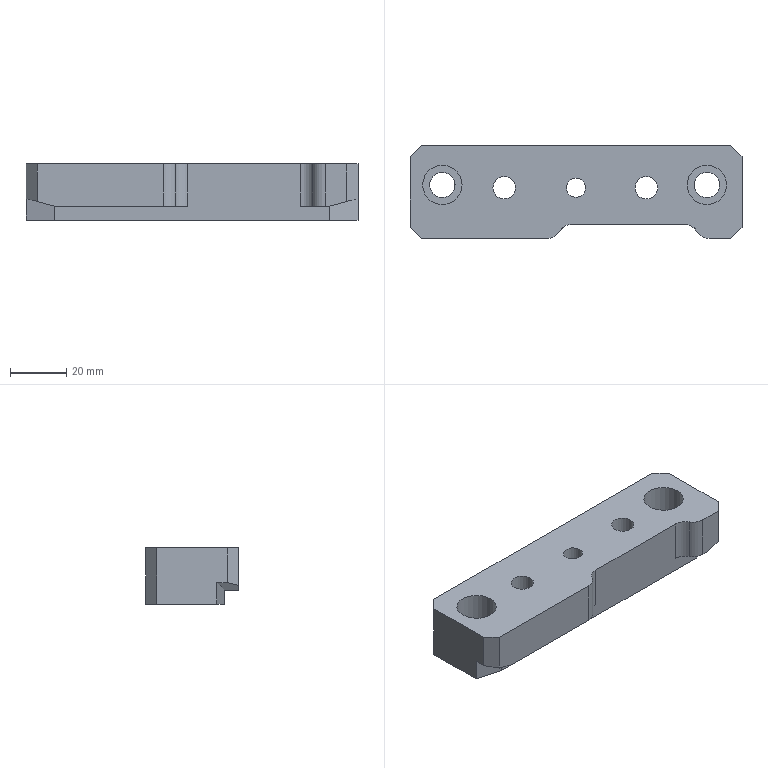Part | NX | features 20 2 | 1 solid | 31 faces | box 118 x 33 x 20 mm | volume 63338 mm3 | plane 20 | cylinder 11 | commonest cylinder face diameters 10 x4 8.001 x2 9 x2 14 x2 6.8 x1
STEP:
#1=CARTESIAN_POINT('',(771.502,417.5,1.5));
#2=VERTEX_POINT('',#1);
#3=CARTESIAN_POINT('',(771.502,422.5,1.5));
#4=VERTEX_POINT('',#3);
#5=CARTESIAN_POINT('',(771.502,417.5,1.5));
#6=DIRECTION('',(0.,1.,0.));
#7=VECTOR('',#6,1000.);
#8=LINE('',#5,#7);
#9=EDGE_CURVE('',#2,#4,#8,.T.);
#10=ORIENTED_EDGE('',*,*,#9,.T.);
#11=CARTESIAN_POINT('',(818.929,422.5,1.5));
#12=VERTEX_POINT('',#11);
#13=CARTESIAN_POINT('',(698.,422.5,1.5));
#14=DIRECTION('',(-1.,0.,0.));
#15=VECTOR('',#14,1000.);
#16=LINE('',#13,#15);
#17=EDGE_CURVE('',#12,#4,#16,.T.);
#18=ORIENTED_EDGE('',*,*,#17,.F.);
#19=CARTESIAN_POINT('',(814.598,420.,1.5));
#20=VERTEX_POINT('',#19);
#21=CARTESIAN_POINT('',(818.929,417.5,1.5));
#22=DIRECTION('',(0.,0.,-1.));
#23=DIRECTION('',(-1.,0.,0.));
#24=AXIS2_PLACEMENT_3D('',#21,#22,#23);
#25=CIRCLE('',#24,5.);
#26=EDGE_CURVE('',#20,#12,#25,.T.);
#27=ORIENTED_EDGE('',*,*,#26,.F.);
#28=CARTESIAN_POINT('',(810.268,417.5,1.5));
#29=VERTEX_POINT('',#28);
#30=CARTESIAN_POINT('',(810.268,422.5,1.5));
#31=DIRECTION('',(0.,0.,-1.));
#32=DIRECTION('',(-1.,0.,0.));
#33=AXIS2_PLACEMENT_3D('',#30,#31,#32);
#34=CIRCLE('',#33,5.);
#35=EDGE_CURVE('',#20,#29,#34,.T.);
#36=ORIENTED_EDGE('',*,*,#35,.T.);
#37=CARTESIAN_POINT('',(708.002,417.5,1.5));
#38=DIRECTION('',(-1.,0.,0.));
#39=VECTOR('',#38,1000.);
#40=LINE('',#37,#39);
#41=EDGE_CURVE('',#29,#2,#40,.T.);
#42=ORIENTED_EDGE('',*,*,#41,.T.);
#43=EDGE_LOOP('',(#10,#18,#27,#36,#42));
#44=FACE_BOUND('',#43,.T.);
#45=CARTESIAN_POINT('',(730.272,396.891,1.5));
#46=DIRECTION('',(0.,0.,-1.));
#47=DIRECTION('',(1.,0.,0.));
#48=AXIS2_PLACEMENT_3D('',#45,#46,#47);
#49=PLANE('',#48);
#50=ADVANCED_FACE('',(#44),#49,.T.);
#51=CARTESIAN_POINT('',(863.459,420.,1.5));
#52=VERTEX_POINT('',#51);
#53=CARTESIAN_POINT('',(859.129,422.5,1.5));
#54=VERTEX_POINT('',#53);
#55=CARTESIAN_POINT('',(859.129,417.5,1.5));
#56=DIRECTION('',(0.,0.,1.));
#57=DIRECTION('',(-1.,0.,0.));
#58=AXIS2_PLACEMENT_3D('',#55,#56,#57);
#59=CIRCLE('',#58,5.);
#60=EDGE_CURVE('',#52,#54,#59,.T.);
#61=ORIENTED_EDGE('',*,*,#60,.T.);
#62=CARTESIAN_POINT('',(869.503,422.5,1.5));
#63=VERTEX_POINT('',#62);
#64=CARTESIAN_POINT('',(698.,422.5,1.5));
#65=DIRECTION('',(-1.,0.,0.));
#66=VECTOR('',#65,1000.);
#67=LINE('',#64,#66);
#68=EDGE_CURVE('',#63,#54,#67,.T.);
#69=ORIENTED_EDGE('',*,*,#68,.F.);
#70=CARTESIAN_POINT('',(869.502,422.5,1.5));
#71=VERTEX_POINT('',#70);
#72=CARTESIAN_POINT('',(733.197,385.977,1.5));
#73=DIRECTION('',(0.9659,0.2588,0.));
#74=VECTOR('',#73,1000.);
#75=LINE('',#72,#74);
#76=EDGE_CURVE('',#71,#63,#75,.T.);
#77=ORIENTED_EDGE('',*,*,#76,.F.);
#78=CARTESIAN_POINT('',(869.502,417.5,1.5));
#79=VERTEX_POINT('',#78);
#80=CARTESIAN_POINT('',(869.502,396.891,1.5));
#81=DIRECTION('',(0.,1.,0.));
#82=VECTOR('',#81,1000.);
#83=LINE('',#80,#82);
#84=EDGE_CURVE('',#79,#71,#83,.T.);
#85=ORIENTED_EDGE('',*,*,#84,.F.);
#86=CARTESIAN_POINT('',(867.789,417.5,1.5));
#87=VERTEX_POINT('',#86);
#88=CARTESIAN_POINT('',(689.002,417.5,1.5));
#89=DIRECTION('',(-1.,0.,0.));
#90=VECTOR('',#89,1000.);
#91=LINE('',#88,#90);
#92=EDGE_CURVE('',#79,#87,#91,.T.);
#93=ORIENTED_EDGE('',*,*,#92,.T.);
#94=CARTESIAN_POINT('',(867.789,422.5,1.5));
#95=DIRECTION('',(0.,0.,1.));
#96=DIRECTION('',(-1.,0.,0.));
#97=AXIS2_PLACEMENT_3D('',#94,#95,#96);
#98=CIRCLE('',#97,5.);
#99=EDGE_CURVE('',#52,#87,#98,.T.);
#100=ORIENTED_EDGE('',*,*,#99,.F.);
#101=EDGE_LOOP('',(#61,#69,#77,#85,#93,#100));
#102=FACE_BOUND('',#101,.T.);
#103=CARTESIAN_POINT('',(730.272,396.891,1.5));
#104=DIRECTION('',(0.,0.,-1.));
#105=DIRECTION('',(1.,0.,0.));
#106=AXIS2_PLACEMENT_3D('',#103,#104,#105);
#107=PLANE('',#106);
#108=ADVANCED_FACE('',(#102),#107,.T.);
#109=CARTESIAN_POINT('',(875.502,417.5,3.108));
#110=VERTEX_POINT('',#109);
#111=CARTESIAN_POINT('',(869.502,417.5,1.5));
#112=DIRECTION('',(0.9659,0.,0.2588));
#113=VECTOR('',#112,1000.);
#114=LINE('',#111,#113);
#115=EDGE_CURVE('',#79,#110,#114,.T.);
#116=ORIENTED_EDGE('',*,*,#115,.F.);
#117=ORIENTED_EDGE('',*,*,#84,.T.);
#118=CARTESIAN_POINT('',(879.502,425.179,4.179));
#119=VERTEX_POINT('',#118);
#120=CARTESIAN_POINT('',(869.971,422.626,1.626));
#121=DIRECTION('',(-0.9351,-0.2506,-0.2506));
#122=VECTOR('',#121,1000.);
#123=LINE('',#120,#122);
#124=EDGE_CURVE('',#119,#71,#123,.T.);
#125=ORIENTED_EDGE('',*,*,#124,.F.);
#126=CARTESIAN_POINT('',(879.502,421.5,4.179));
#127=VERTEX_POINT('',#126);
#128=CARTESIAN_POINT('',(879.502,396.891,4.179));
#129=DIRECTION('',(0.,1.,0.));
#130=VECTOR('',#129,1000.);
#131=LINE('',#128,#130);
#132=EDGE_CURVE('',#127,#119,#131,.T.);
#133=ORIENTED_EDGE('',*,*,#132,.F.);
#134=CARTESIAN_POINT('',(876.587,418.585,3.399));
#135=DIRECTION('',(-0.6947,-0.6947,-0.1862));
#136=VECTOR('',#135,1000.);
#137=LINE('',#134,#136);
#138=EDGE_CURVE('',#127,#110,#137,.T.);
#139=ORIENTED_EDGE('',*,*,#138,.T.);
#140=EDGE_LOOP('',(#116,#117,#125,#133,#139));
#141=FACE_BOUND('',#140,.T.);
#142=CARTESIAN_POINT('',(869.502,396.891,1.5));
#143=DIRECTION('',(0.2588,0.,-0.9659));
#144=DIRECTION('',(-0.9659,0.,-0.2588));
#145=AXIS2_PLACEMENT_3D('',#142,#143,#144);
#146=PLANE('',#145);
#147=ADVANCED_FACE('',(#141),#146,.T.);
#148=CARTESIAN_POINT('',(799.002,435.5,-3.5));
#149=VERTEX_POINT('',#148);
#150=CARTESIAN_POINT('',(795.002,435.5,-3.5));
#151=DIRECTION('',(0.,0.,-1.));
#152=DIRECTION('',(1.,0.,0.));
#153=AXIS2_PLACEMENT_3D('',#150,#151,#152);
#154=CIRCLE('',#153,4.);
#155=EDGE_CURVE('',#149,#149,#154,.T.);
#156=ORIENTED_EDGE('',*,*,#155,.T.);
#157=EDGE_LOOP('',(#156));
#158=FACE_BOUND('',#157,.T.);
#159=CARTESIAN_POINT('',(799.002,435.5,16.5));
#160=VERTEX_POINT('',#159);
#161=CARTESIAN_POINT('',(795.002,435.5,16.5));
#162=DIRECTION('',(0.,0.,1.));
#163=DIRECTION('',(1.,0.,0.));
#164=AXIS2_PLACEMENT_3D('',#161,#162,#163);
#165=CIRCLE('',#164,4.);
#166=EDGE_CURVE('',#160,#160,#165,.T.);
#167=ORIENTED_EDGE('',*,*,#166,.T.);
#168=EDGE_LOOP('',(#167));
#169=FACE_BOUND('',#168,.T.);
#170=CARTESIAN_POINT('',(795.002,435.5,42.5));
#171=DIRECTION('',(0.,0.,-1.));
#172=DIRECTION('',(1.,0.,0.));
#173=AXIS2_PLACEMENT_3D('',#170,#171,#172);
#174=CYLINDRICAL_SURFACE('',#173,4.);
#175=ADVANCED_FACE('',(#158,#169),#174,.F.);
#176=CARTESIAN_POINT('',(849.502,435.5,-3.5));
#177=VERTEX_POINT('',#176);
#178=CARTESIAN_POINT('',(845.502,435.5,-3.5));
#179=DIRECTION('',(0.,0.,1.));
#180=DIRECTION('',(1.,0.,0.));
#181=AXIS2_PLACEMENT_3D('',#178,#179,#180);
#182=CIRCLE('',#181,4.);
#183=EDGE_CURVE('',#177,#177,#182,.T.);
#184=ORIENTED_EDGE('',*,*,#183,.F.);
#185=EDGE_LOOP('',(#184));
#186=FACE_BOUND('',#185,.T.);
#187=CARTESIAN_POINT('',(849.502,435.5,16.5));
#188=VERTEX_POINT('',#187);
#189=CARTESIAN_POINT('',(845.502,435.5,16.5));
#190=DIRECTION('',(0.,0.,1.));
#191=DIRECTION('',(1.,0.,0.));
#192=AXIS2_PLACEMENT_3D('',#189,#190,#191);
#193=CIRCLE('',#192,4.);
#194=EDGE_CURVE('',#188,#188,#193,.T.);
#195=ORIENTED_EDGE('',*,*,#194,.T.);
#196=EDGE_LOOP('',(#195));
#197=FACE_BOUND('',#196,.T.);
#198=CARTESIAN_POINT('',(845.502,435.5,42.5));
#199=DIRECTION('',(0.,0.,-1.));
#200=DIRECTION('',(1.,0.,0.));
#201=AXIS2_PLACEMENT_3D('',#198,#199,#200);
#202=CYLINDRICAL_SURFACE('',#201,4.);
#203=ADVANCED_FACE('',(#186,#197),#202,.F.);
#204=CARTESIAN_POINT('',(879.502,425.179,-3.5));
#205=VERTEX_POINT('',#204);
#206=CARTESIAN_POINT('',(879.502,425.179,3.5));
#207=DIRECTION('',(0.,0.,1.));
#208=VECTOR('',#207,1000.);
#209=LINE('',#206,#208);
#210=EDGE_CURVE('',#205,#119,#209,.T.);
#211=ORIENTED_EDGE('',*,*,#210,.F.);
#212=CARTESIAN_POINT('',(879.502,446.5,-3.5));
#213=VERTEX_POINT('',#212);
#214=CARTESIAN_POINT('',(879.502,450.5,-3.5));
#215=DIRECTION('',(0.,1.,0.));
#216=VECTOR('',#215,1000.);
#217=LINE('',#214,#216);
#218=EDGE_CURVE('',#205,#213,#217,.T.);
#219=ORIENTED_EDGE('',*,*,#218,.T.);
#220=CARTESIAN_POINT('',(879.502,446.5,16.5));
#221=VERTEX_POINT('',#220);
#222=CARTESIAN_POINT('',(879.502,446.5,11.5));
#223=DIRECTION('',(0.,0.,1.));
#224=VECTOR('',#223,1000.);
#225=LINE('',#222,#224);
#226=EDGE_CURVE('',#213,#221,#225,.T.);
#227=ORIENTED_EDGE('',*,*,#226,.T.);
#228=CARTESIAN_POINT('',(879.502,421.5,16.5));
#229=VERTEX_POINT('',#228);
#230=CARTESIAN_POINT('',(879.502,450.5,16.5));
#231=DIRECTION('',(0.,1.,0.));
#232=VECTOR('',#231,1000.);
#233=LINE('',#230,#232);
#234=EDGE_CURVE('',#229,#221,#233,.T.);
#235=ORIENTED_EDGE('',*,*,#234,.F.);
#236=CARTESIAN_POINT('',(879.502,421.5,11.5));
#237=DIRECTION('',(0.,0.,-1.));
#238=VECTOR('',#237,1000.);
#239=LINE('',#236,#238);
#240=EDGE_CURVE('',#229,#127,#239,.T.);
#241=ORIENTED_EDGE('',*,*,#240,.T.);
#242=ORIENTED_EDGE('',*,*,#132,.T.);
#243=EDGE_LOOP('',(#211,#219,#227,#235,#241,#242));
#244=FACE_BOUND('',#243,.T.);
#245=CARTESIAN_POINT('',(879.502,450.5,11.5));
#246=DIRECTION('',(-1.,0.,0.));
#247=DIRECTION('',(0.,0.,-1.));
#248=AXIS2_PLACEMENT_3D('',#245,#246,#247);
#249=PLANE('',#248);
#250=ADVANCED_FACE('',(#244),#249,.F.);
#251=ORIENTED_EDGE('',*,*,#226,.F.);
#252=CARTESIAN_POINT('',(875.502,450.5,-3.5));
#253=VERTEX_POINT('',#252);
#254=CARTESIAN_POINT('',(879.502,446.5,-3.5));
#255=DIRECTION('',(0.7071,-0.7071,0.));
#256=VECTOR('',#255,1000.);
#257=LINE('',#254,#256);
#258=EDGE_CURVE('',#253,#213,#257,.T.);
#259=ORIENTED_EDGE('',*,*,#258,.F.);
#260=CARTESIAN_POINT('',(875.502,450.5,16.5));
#261=VERTEX_POINT('',#260);
#262=CARTESIAN_POINT('',(875.502,450.5,11.5));
#263=DIRECTION('',(0.,0.,-1.));
#264=VECTOR('',#263,1000.);
#265=LINE('',#262,#264);
#266=EDGE_CURVE('',#261,#253,#265,.T.);
#267=ORIENTED_EDGE('',*,*,#266,.F.);
#268=CARTESIAN_POINT('',(879.502,446.5,16.5));
#269=DIRECTION('',(-0.7071,0.7071,0.));
#270=VECTOR('',#269,1000.);
#271=LINE('',#268,#270);
#272=EDGE_CURVE('',#221,#261,#271,.T.);
#273=ORIENTED_EDGE('',*,*,#272,.F.);
#274=EDGE_LOOP('',(#251,#259,#267,#273));
#275=FACE_BOUND('',#274,.T.);
#276=CARTESIAN_POINT('',(879.502,446.5,11.5));
#277=DIRECTION('',(-0.7071,-0.7071,0.));
#278=DIRECTION('',(0.,0.,-1.));
#279=AXIS2_PLACEMENT_3D('',#276,#277,#278);
#280=PLANE('',#279);
#281=ADVANCED_FACE('',(#275),#280,.F.);
#282=ORIENTED_EDGE('',*,*,#266,.T.);
#283=CARTESIAN_POINT('',(765.502,450.5,-3.5));
#284=VERTEX_POINT('',#283);
#285=CARTESIAN_POINT('',(628.002,450.5,-3.5));
#286=DIRECTION('',(-1.,0.,0.));
#287=VECTOR('',#286,1000.);
#288=LINE('',#285,#287);
#289=EDGE_CURVE('',#253,#284,#288,.T.);
#290=ORIENTED_EDGE('',*,*,#289,.T.);
#291=CARTESIAN_POINT('',(765.502,450.5,16.5));
#292=VERTEX_POINT('',#291);
#293=CARTESIAN_POINT('',(765.502,450.5,11.5));
#294=DIRECTION('',(0.,0.,1.));
#295=VECTOR('',#294,1000.);
#296=LINE('',#293,#295);
#297=EDGE_CURVE('',#284,#292,#296,.T.);
#298=ORIENTED_EDGE('',*,*,#297,.T.);
#299=CARTESIAN_POINT('',(628.002,450.5,16.5));
#300=DIRECTION('',(-1.,0.,0.));
#301=VECTOR('',#300,1000.);
#302=LINE('',#299,#301);
#303=EDGE_CURVE('',#261,#292,#302,.T.);
#304=ORIENTED_EDGE('',*,*,#303,.F.);
#305=EDGE_LOOP('',(#282,#290,#298,#304));
#306=FACE_BOUND('',#305,.T.);
#307=CARTESIAN_POINT('',(628.002,450.5,11.5));
#308=DIRECTION('',(0.,-1.,0.));
#309=DIRECTION('',(0.,0.,-1.));
#310=AXIS2_PLACEMENT_3D('',#307,#308,#309);
#311=PLANE('',#310);
#312=ADVANCED_FACE('',(#306),#311,.F.);
#313=ORIENTED_EDGE('',*,*,#297,.F.);
#314=CARTESIAN_POINT('',(761.502,446.5,-3.5));
#315=VERTEX_POINT('',#314);
#316=CARTESIAN_POINT('',(765.502,450.5,-3.5));
#317=DIRECTION('',(0.7071,0.7071,0.));
#318=VECTOR('',#317,1000.);
#319=LINE('',#316,#318);
#320=EDGE_CURVE('',#315,#284,#319,.T.);
#321=ORIENTED_EDGE('',*,*,#320,.F.);
#322=CARTESIAN_POINT('',(761.502,446.5,16.5));
#323=VERTEX_POINT('',#322);
#324=CARTESIAN_POINT('',(761.502,446.5,11.5));
#325=DIRECTION('',(0.,0.,-1.));
#326=VECTOR('',#325,1000.);
#327=LINE('',#324,#326);
#328=EDGE_CURVE('',#323,#315,#327,.T.);
#329=ORIENTED_EDGE('',*,*,#328,.F.);
#330=CARTESIAN_POINT('',(765.502,450.5,16.5));
#331=DIRECTION('',(-0.7071,-0.7071,0.));
#332=VECTOR('',#331,1000.);
#333=LINE('',#330,#332);
#334=EDGE_CURVE('',#292,#323,#333,.T.);
#335=ORIENTED_EDGE('',*,*,#334,.F.);
#336=EDGE_LOOP('',(#313,#321,#329,#335));
#337=FACE_BOUND('',#336,.T.);
#338=CARTESIAN_POINT('',(765.502,450.5,11.5));
#339=DIRECTION('',(0.7071,-0.7071,0.));
#340=DIRECTION('',(0.,0.,-1.));
#341=AXIS2_PLACEMENT_3D('',#338,#339,#340);
#342=PLANE('',#341);
#343=ADVANCED_FACE('',(#337),#342,.F.);
#344=ORIENTED_EDGE('',*,*,#328,.T.);
#345=CARTESIAN_POINT('',(761.502,425.179,-3.5));
#346=VERTEX_POINT('',#345);
#347=CARTESIAN_POINT('',(761.502,417.5,-3.5));
#348=DIRECTION('',(0.,-1.,0.));
#349=VECTOR('',#348,1000.);
#350=LINE('',#347,#349);
#351=EDGE_CURVE('',#315,#346,#350,.T.);
#352=ORIENTED_EDGE('',*,*,#351,.T.);
#353=CARTESIAN_POINT('',(761.502,425.179,4.179));
#354=VERTEX_POINT('',#353);
#355=CARTESIAN_POINT('',(761.502,425.179,3.5));
#356=DIRECTION('',(0.,0.,1.));
#357=VECTOR('',#356,1000.);
#358=LINE('',#355,#357);
#359=EDGE_CURVE('',#346,#354,#358,.T.);
#360=ORIENTED_EDGE('',*,*,#359,.T.);
#361=CARTESIAN_POINT('',(761.502,421.5,4.179));
#362=VERTEX_POINT('',#361);
#363=CARTESIAN_POINT('',(761.502,425.179,4.179));
#364=DIRECTION('',(0.,-1.,0.));
#365=VECTOR('',#364,1000.);
#366=LINE('',#363,#365);
#367=EDGE_CURVE('',#354,#362,#366,.T.);
#368=ORIENTED_EDGE('',*,*,#367,.T.);
#369=CARTESIAN_POINT('',(761.502,421.5,16.5));
#370=VERTEX_POINT('',#369);
#371=CARTESIAN_POINT('',(761.502,421.5,11.5));
#372=DIRECTION('',(0.,0.,1.));
#373=VECTOR('',#372,1000.);
#374=LINE('',#371,#373);
#375=EDGE_CURVE('',#362,#370,#374,.T.);
#376=ORIENTED_EDGE('',*,*,#375,.T.);
#377=CARTESIAN_POINT('',(761.502,417.5,16.5));
#378=DIRECTION('',(0.,-1.,0.));
#379=VECTOR('',#378,1000.);
#380=LINE('',#377,#379);
#381=EDGE_CURVE('',#323,#370,#380,.T.);
#382=ORIENTED_EDGE('',*,*,#381,.F.);
#383=EDGE_LOOP('',(#344,#352,#360,#368,#376,#382));
#384=FACE_BOUND('',#383,.T.);
#385=CARTESIAN_POINT('',(761.502,417.5,11.5));
#386=DIRECTION('',(1.,0.,0.));
#387=DIRECTION('',(0.,0.,1.));
#388=AXIS2_PLACEMENT_3D('',#385,#386,#387);
#389=PLANE('',#388);
#390=ADVANCED_FACE('',(#384),#389,.F.);
#391=ORIENTED_EDGE('',*,*,#92,.F.);
#392=ORIENTED_EDGE('',*,*,#115,.T.);
#393=CARTESIAN_POINT('',(875.502,417.5,16.5));
#394=VERTEX_POINT('',#393);
#395=CARTESIAN_POINT('',(875.502,417.5,11.5));
#396=DIRECTION('',(0.,0.,1.));
#397=VECTOR('',#396,1000.);
#398=LINE('',#395,#397);
#399=EDGE_CURVE('',#110,#394,#398,.T.);
#400=ORIENTED_EDGE('',*,*,#399,.T.);
#401=CARTESIAN_POINT('',(867.789,417.5,16.5));
#402=VERTEX_POINT('',#401);
#403=CARTESIAN_POINT('',(689.002,417.5,16.5));
#404=DIRECTION('',(1.,0.,0.));
#405=VECTOR('',#404,1000.);
#406=LINE('',#403,#405);
#407=EDGE_CURVE('',#402,#394,#406,.T.);
#408=ORIENTED_EDGE('',*,*,#407,.F.);
#409=CARTESIAN_POINT('',(867.789,417.5,6.5));
#410=DIRECTION('',(0.,0.,-1.));
#411=VECTOR('',#410,1000.);
#412=LINE('',#409,#411);
#413=EDGE_CURVE('',#402,#87,#412,.T.);
#414=ORIENTED_EDGE('',*,*,#413,.T.);
#415=EDGE_LOOP('',(#391,#392,#400,#408,#414));
#416=FACE_BOUND('',#415,.T.);
#417=CARTESIAN_POINT('',(689.002,417.5,11.5));
#418=DIRECTION('',(0.,1.,0.));
#419=DIRECTION('',(0.,0.,1.));
#420=AXIS2_PLACEMENT_3D('',#417,#418,#419);
#421=PLANE('',#420);
#422=ADVANCED_FACE('',(#416),#421,.F.);
#423=ORIENTED_EDGE('',*,*,#76,.T.);
#424=CARTESIAN_POINT('',(869.503,422.5,-3.5));
#425=VERTEX_POINT('',#424);
#426=CARTESIAN_POINT('',(869.503,422.5,3.5));
#427=DIRECTION('',(0.,0.,-1.));
#428=VECTOR('',#427,1000.);
#429=LINE('',#426,#428);
#430=EDGE_CURVE('',#63,#425,#429,.T.);
#431=ORIENTED_EDGE('',*,*,#430,.T.);
#432=CARTESIAN_POINT('',(869.503,422.5,-3.5));
#433=DIRECTION('',(0.9659,0.2588,0.));
#434=VECTOR('',#433,1000.);
#435=LINE('',#432,#434);
#436=EDGE_CURVE('',#425,#205,#435,.T.);
#437=ORIENTED_EDGE('',*,*,#436,.T.);
#438=ORIENTED_EDGE('',*,*,#210,.T.);
#439=ORIENTED_EDGE('',*,*,#124,.T.);
#440=EDGE_LOOP('',(#423,#431,#437,#438,#439));
#441=FACE_BOUND('',#440,.T.);
#442=CARTESIAN_POINT('',(869.503,422.5,3.5));
#443=DIRECTION('',(-0.2588,0.9659,0.));
#444=DIRECTION('',(-0.9659,-0.2588,0.));
#445=AXIS2_PLACEMENT_3D('',#442,#443,#444);
#446=PLANE('',#445);
#447=ADVANCED_FACE('',(#441),#446,.F.);
#448=CARTESIAN_POINT('',(818.929,422.5,16.5));
#449=VERTEX_POINT('',#448);
#450=CARTESIAN_POINT('',(818.929,422.5,3.5));
#451=DIRECTION('',(0.,0.,1.));
#452=VECTOR('',#451,1000.);
#453=LINE('',#450,#452);
#454=EDGE_CURVE('',#12,#449,#453,.T.);
#455=ORIENTED_EDGE('',*,*,#454,.F.);
#456=ORIENTED_EDGE('',*,*,#17,.T.);
#457=CARTESIAN_POINT('',(771.501,422.5,1.5));
#458=VERTEX_POINT('',#457);
#459=CARTESIAN_POINT('',(827.481,422.5,-13.5));
#460=DIRECTION('',(-0.9659,0.,0.2588));
#461=VECTOR('',#460,1000.);
#462=LINE('',#459,#461);
#463=EDGE_CURVE('',#4,#458,#462,.T.);
#464=ORIENTED_EDGE('',*,*,#463,.T.);
#465=CARTESIAN_POINT('',(771.501,422.5,-3.5));
#466=VERTEX_POINT('',#465);
#467=CARTESIAN_POINT('',(771.501,422.5,3.5));
#468=DIRECTION('',(0.,0.,-1.));
#469=VECTOR('',#468,1000.);
#470=LINE('',#467,#469);
#471=EDGE_CURVE('',#458,#466,#470,.T.);
#472=ORIENTED_EDGE('',*,*,#471,.T.);
#473=CARTESIAN_POINT('',(698.,422.5,-3.5));
#474=DIRECTION('',(1.,0.,0.));
#475=VECTOR('',#474,1000.);
#476=LINE('',#473,#475);
#477=EDGE_CURVE('',#466,#425,#476,.T.);
#478=ORIENTED_EDGE('',*,*,#477,.T.);
#479=ORIENTED_EDGE('',*,*,#430,.F.);
#480=ORIENTED_EDGE('',*,*,#68,.T.);
#481=CARTESIAN_POINT('',(859.129,422.5,16.5));
#482=VERTEX_POINT('',#481);
#483=CARTESIAN_POINT('',(859.129,422.5,3.5));
#484=DIRECTION('',(0.,0.,-1.));
#485=VECTOR('',#484,1000.);
#486=LINE('',#483,#485);
#487=EDGE_CURVE('',#482,#54,#486,.T.);
#488=ORIENTED_EDGE('',*,*,#487,.F.);
#489=CARTESIAN_POINT('',(708.002,422.5,16.5));
#490=DIRECTION('',(-1.,0.,0.));
#491=VECTOR('',#490,1000.);
#492=LINE('',#489,#491);
#493=EDGE_CURVE('',#482,#449,#492,.T.);
#494=ORIENTED_EDGE('',*,*,#493,.T.);
#495=EDGE_LOOP('',(#455,#456,#464,#472,#478,#479,#480,#488,#494));
#496=FACE_BOUND('',#495,.T.);
#497=CARTESIAN_POINT('',(698.,422.5,3.5));
#498=DIRECTION('',(0.,1.,0.));
#499=DIRECTION('',(0.,0.,1.));
#500=AXIS2_PLACEMENT_3D('',#497,#498,#499);
#501=PLANE('',#500);
#502=ADVANCED_FACE('',(#496),#501,.F.);
#503=ORIENTED_EDGE('',*,*,#359,.F.);
#504=CARTESIAN_POINT('',(771.501,422.5,-3.5));
#505=DIRECTION('',(0.9659,-0.2588,0.));
#506=VECTOR('',#505,1000.);
#507=LINE('',#504,#506);
#508=EDGE_CURVE('',#346,#466,#507,.T.);
#509=ORIENTED_EDGE('',*,*,#508,.T.);
#510=ORIENTED_EDGE('',*,*,#471,.F.);
#511=CARTESIAN_POINT('',(771.501,422.5,1.5));
#512=DIRECTION('',(-0.9351,0.2506,0.2506));
#513=VECTOR('',#512,1000.);
#514=LINE('',#511,#513);
#515=EDGE_CURVE('',#458,#354,#514,.T.);
#516=ORIENTED_EDGE('',*,*,#515,.T.);
#517=EDGE_LOOP('',(#503,#509,#510,#516));
#518=FACE_BOUND('',#517,.T.);
#519=CARTESIAN_POINT('',(771.501,422.5,3.5));
#520=DIRECTION('',(0.2588,0.9659,0.));
#521=DIRECTION('',(0.9659,-0.2588,0.));
#522=AXIS2_PLACEMENT_3D('',#519,#520,#521);
#523=PLANE('',#522);
#524=ADVANCED_FACE('',(#518),#523,.F.);
#525=CARTESIAN_POINT('',(823.902,435.5,16.5));
#526=VERTEX_POINT('',#525);
#527=CARTESIAN_POINT('',(820.502,435.5,16.5));
#528=DIRECTION('',(0.,0.,-1.));
#529=DIRECTION('',(1.,0.,0.));
#530=AXIS2_PLACEMENT_3D('',#527,#528,#529);
#531=CIRCLE('',#530,3.4);
#532=EDGE_CURVE('',#526,#526,#531,.T.);
#533=ORIENTED_EDGE('',*,*,#532,.F.);
#534=EDGE_LOOP('',(#533));
#535=FACE_BOUND('',#534,.T.);
#536=CARTESIAN_POINT('',(823.902,435.5,-3.5));
#537=VERTEX_POINT('',#536);
#538=CARTESIAN_POINT('',(820.502,435.5,-3.5));
#539=DIRECTION('',(0.,0.,-1.));
#540=DIRECTION('',(1.,0.,0.));
#541=AXIS2_PLACEMENT_3D('',#538,#539,#540);
#542=CIRCLE('',#541,3.4);
#543=EDGE_CURVE('',#537,#537,#542,.T.);
#544=ORIENTED_EDGE('',*,*,#543,.T.);
#545=EDGE_LOOP('',(#544));
#546=FACE_BOUND('',#545,.T.);
#547=CARTESIAN_POINT('',(820.502,435.5,-671.5));
#548=DIRECTION('',(0.,0.,1.));
#549=DIRECTION('',(1.,0.,0.));
#550=AXIS2_PLACEMENT_3D('',#547,#548,#549);
#551=CYLINDRICAL_SURFACE('',#550,3.4);
#552=ADVANCED_FACE('',(#535,#546),#551,.F.);
#553=ORIENTED_EDGE('',*,*,#60,.F.);
#554=CARTESIAN_POINT('',(863.459,420.,16.5));
#555=VERTEX_POINT('',#554);
#556=CARTESIAN_POINT('',(863.459,420.,-10.));
#557=DIRECTION('',(0.,0.,1.));
#558=VECTOR('',#557,1000.);
#559=LINE('',#556,#558);
#560=EDGE_CURVE('',#52,#555,#559,.T.);
#561=ORIENTED_EDGE('',*,*,#560,.T.);
#562=CARTESIAN_POINT('',(859.129,417.5,16.5));
#563=DIRECTION('',(0.,0.,1.));
#564=DIRECTION('',(1.,0.,0.));
#565=AXIS2_PLACEMENT_3D('',#562,#563,#564);
#566=CIRCLE('',#565,5.);
#567=EDGE_CURVE('',#555,#482,#566,.T.);
#568=ORIENTED_EDGE('',*,*,#567,.T.);
#569=ORIENTED_EDGE('',*,*,#487,.T.);
#570=EDGE_LOOP('',(#553,#561,#568,#569));
#571=FACE_BOUND('',#570,.T.);
#572=CARTESIAN_POINT('',(859.129,417.5,-10.));
#573=DIRECTION('',(0.,0.,1.));
#574=DIRECTION('',(-1.,0.,0.));
#575=AXIS2_PLACEMENT_3D('',#572,#573,#574);
#576=CYLINDRICAL_SURFACE('',#575,5.);
#577=ADVANCED_FACE('',(#571),#576,.F.);
#578=ORIENTED_EDGE('',*,*,#560,.F.);
#579=ORIENTED_EDGE('',*,*,#99,.T.);
#580=ORIENTED_EDGE('',*,*,#413,.F.);
#581=CARTESIAN_POINT('',(867.789,422.5,16.5));
#582=DIRECTION('',(0.,0.,1.));
#583=DIRECTION('',(1.,0.,0.));
#584=AXIS2_PLACEMENT_3D('',#581,#582,#583);
#585=CIRCLE('',#584,5.);
#586=EDGE_CURVE('',#555,#402,#585,.T.);
#587=ORIENTED_EDGE('',*,*,#586,.F.);
#588=EDGE_LOOP('',(#578,#579,#580,#587));
#589=FACE_BOUND('',#588,.T.);
#590=CARTESIAN_POINT('',(867.789,422.5,-10.));
#591=DIRECTION('',(0.,0.,1.));
#592=DIRECTION('',(-1.,0.,0.));
#593=AXIS2_PLACEMENT_3D('',#590,#591,#592);
#594=CYLINDRICAL_SURFACE('',#593,5.);
#595=ADVANCED_FACE('',(#589),#594,.T.);
#596=ORIENTED_EDGE('',*,*,#41,.F.);
#597=CARTESIAN_POINT('',(810.268,417.5,16.5));
#598=VERTEX_POINT('',#597);
#599=CARTESIAN_POINT('',(810.268,417.5,11.5));
#600=DIRECTION('',(0.,0.,1.));
#601=VECTOR('',#600,1000.);
#602=LINE('',#599,#601);
#603=EDGE_CURVE('',#29,#598,#602,.T.);
#604=ORIENTED_EDGE('',*,*,#603,.T.);
#605=CARTESIAN_POINT('',(765.502,417.5,16.5));
#606=VERTEX_POINT('',#605);
#607=CARTESIAN_POINT('',(708.002,417.5,16.5));
#608=DIRECTION('',(1.,0.,0.));
#609=VECTOR('',#608,1000.);
#610=LINE('',#607,#609);
#611=EDGE_CURVE('',#606,#598,#610,.T.);
#612=ORIENTED_EDGE('',*,*,#611,.F.);
#613=CARTESIAN_POINT('',(765.502,417.5,3.108));
#614=VERTEX_POINT('',#613);
#615=CARTESIAN_POINT('',(765.502,417.5,11.5));
#616=DIRECTION('',(0.,0.,-1.));
#617=VECTOR('',#616,1000.);
#618=LINE('',#615,#617);
#619=EDGE_CURVE('',#606,#614,#618,.T.);
#620=ORIENTED_EDGE('',*,*,#619,.T.);
#621=CARTESIAN_POINT('',(771.502,417.5,1.5));
#622=DIRECTION('',(0.9659,0.,-0.2588));
#623=VECTOR('',#622,1000.);
#624=LINE('',#621,#623);
#625=EDGE_CURVE('',#614,#2,#624,.T.);
#626=ORIENTED_EDGE('',*,*,#625,.T.);
#627=EDGE_LOOP('',(#596,#604,#612,#620,#626));
#628=FACE_BOUND('',#627,.T.);
#629=CARTESIAN_POINT('',(708.002,417.5,11.5));
#630=DIRECTION('',(0.,1.,0.));
#631=DIRECTION('',(0.,0.,1.));
#632=AXIS2_PLACEMENT_3D('',#629,#630,#631);
#633=PLANE('',#632);
#634=ADVANCED_FACE('',(#628),#633,.F.);
#635=CARTESIAN_POINT('',(780.002,436.5,16.5));
#636=VERTEX_POINT('',#635);
#637=CARTESIAN_POINT('',(773.002,436.5,16.5));
#638=DIRECTION('',(0.,0.,1.));
#639=DIRECTION('',(1.,0.,0.));
#640=AXIS2_PLACEMENT_3D('',#637,#638,#639);
#641=CIRCLE('',#640,7.);
#642=EDGE_CURVE('',#636,#636,#641,.T.);
#643=ORIENTED_EDGE('',*,*,#642,.T.);
#644=EDGE_LOOP('',(#643));
#645=FACE_BOUND('',#644,.T.);
#646=CARTESIAN_POINT('',(780.002,436.5,6.5));
#647=VERTEX_POINT('',#646);
#648=CARTESIAN_POINT('',(773.002,436.5,6.5));
#649=DIRECTION('',(0.,0.,1.));
#650=DIRECTION('',(1.,0.,0.));
#651=AXIS2_PLACEMENT_3D('',#648,#649,#650);
#652=CIRCLE('',#651,7.);
#653=EDGE_CURVE('',#647,#647,#652,.T.);
#654=ORIENTED_EDGE('',*,*,#653,.F.);
#655=EDGE_LOOP('',(#654));
#656=FACE_BOUND('',#655,.T.);
#657=CARTESIAN_POINT('',(773.002,436.5,11.5));
#658=DIRECTION('',(0.,0.,-1.));
#659=DIRECTION('',(-1.,0.,0.));
#660=AXIS2_PLACEMENT_3D('',#657,#658,#659);
#661=CYLINDRICAL_SURFACE('',#660,7.);
#662=ADVANCED_FACE('',(#645,#656),#661,.F.);
#663=CARTESIAN_POINT('',(874.002,436.5,16.5));
#664=VERTEX_POINT('',#663);
#665=CARTESIAN_POINT('',(867.002,436.5,16.5));
#666=DIRECTION('',(0.,0.,-1.));
#667=DIRECTION('',(1.,0.,0.));
#668=AXIS2_PLACEMENT_3D('',#665,#666,#667);
#669=CIRCLE('',#668,7.);
#670=EDGE_CURVE('',#664,#664,#669,.T.);
#671=ORIENTED_EDGE('',*,*,#670,.F.);
#672=EDGE_LOOP('',(#671));
#673=FACE_BOUND('',#672,.T.);
#674=CARTESIAN_POINT('',(874.002,436.5,6.5));
#675=VERTEX_POINT('',#674);
#676=CARTESIAN_POINT('',(867.002,436.5,6.5));
#677=DIRECTION('',(0.,0.,1.));
#678=DIRECTION('',(1.,0.,0.));
#679=AXIS2_PLACEMENT_3D('',#676,#677,#678);
#680=CIRCLE('',#679,7.);
#681=EDGE_CURVE('',#675,#675,#680,.T.);
#682=ORIENTED_EDGE('',*,*,#681,.F.);
#683=EDGE_LOOP('',(#682));
#684=FACE_BOUND('',#683,.T.);
#685=CARTESIAN_POINT('',(867.002,436.5,11.5));
#686=DIRECTION('',(0.,0.,-1.));
#687=DIRECTION('',(-1.,0.,0.));
#688=AXIS2_PLACEMENT_3D('',#685,#686,#687);
#689=CYLINDRICAL_SURFACE('',#688,7.);
#690=ADVANCED_FACE('',(#673,#684),#689,.F.);
#691=ORIENTED_EDGE('',*,*,#399,.F.);
#692=ORIENTED_EDGE('',*,*,#138,.F.);
#693=ORIENTED_EDGE('',*,*,#240,.F.);
#694=CARTESIAN_POINT('',(875.502,417.5,16.5));
#695=DIRECTION('',(0.7071,0.7071,0.));
#696=VECTOR('',#695,1000.);
#697=LINE('',#694,#696);
#698=EDGE_CURVE('',#394,#229,#697,.T.);
#699=ORIENTED_EDGE('',*,*,#698,.F.);
#700=EDGE_LOOP('',(#691,#692,#693,#699));
#701=FACE_BOUND('',#700,.T.);
#702=CARTESIAN_POINT('',(875.502,417.5,11.5));
#703=DIRECTION('',(-0.7071,0.7071,0.));
#704=DIRECTION('',(0.,0.,-1.));
#705=AXIS2_PLACEMENT_3D('',#702,#703,#704);
#706=PLANE('',#705);
#707=ADVANCED_FACE('',(#701),#706,.F.);
#708=ORIENTED_EDGE('',*,*,#375,.F.);
#709=CARTESIAN_POINT('',(778.553,404.449,-0.3894));
#710=DIRECTION('',(-0.6947,0.6947,0.1862));
#711=VECTOR('',#710,1000.);
#712=LINE('',#709,#711);
#713=EDGE_CURVE('',#614,#362,#712,.T.);
#714=ORIENTED_EDGE('',*,*,#713,.F.);
#715=ORIENTED_EDGE('',*,*,#619,.F.);
#716=CARTESIAN_POINT('',(761.502,421.5,16.5));
#717=DIRECTION('',(0.7071,-0.7071,0.));
#718=VECTOR('',#717,1000.);
#719=LINE('',#716,#718);
#720=EDGE_CURVE('',#370,#606,#719,.T.);
#721=ORIENTED_EDGE('',*,*,#720,.F.);
#722=EDGE_LOOP('',(#708,#714,#715,#721));
#723=FACE_BOUND('',#722,.T.);
#724=CARTESIAN_POINT('',(761.502,421.5,11.5));
#725=DIRECTION('',(0.7071,0.7071,0.));
#726=DIRECTION('',(0.,0.,-1.));
#727=AXIS2_PLACEMENT_3D('',#724,#725,#726);
#728=PLANE('',#727);
#729=ADVANCED_FACE('',(#723),#728,.F.);
#730=ORIENTED_EDGE('',*,*,#166,.F.);
#731=EDGE_LOOP('',(#730));
#732=FACE_BOUND('',#731,.T.);
#733=ORIENTED_EDGE('',*,*,#194,.F.);
#734=EDGE_LOOP('',(#733));
#735=FACE_BOUND('',#734,.T.);
#736=ORIENTED_EDGE('',*,*,#611,.T.);
#737=CARTESIAN_POINT('',(814.598,420.,16.5));
#738=VERTEX_POINT('',#737);
#739=CARTESIAN_POINT('',(810.268,422.5,16.5));
#740=DIRECTION('',(0.,0.,1.));
#741=DIRECTION('',(1.,0.,0.));
#742=AXIS2_PLACEMENT_3D('',#739,#740,#741);
#743=CIRCLE('',#742,5.);
#744=EDGE_CURVE('',#598,#738,#743,.T.);
#745=ORIENTED_EDGE('',*,*,#744,.T.);
#746=CARTESIAN_POINT('',(818.929,417.5,16.5));
#747=DIRECTION('',(0.,0.,1.));
#748=DIRECTION('',(1.,0.,0.));
#749=AXIS2_PLACEMENT_3D('',#746,#747,#748);
#750=CIRCLE('',#749,5.);
#751=EDGE_CURVE('',#449,#738,#750,.T.);
#752=ORIENTED_EDGE('',*,*,#751,.F.);
#753=ORIENTED_EDGE('',*,*,#493,.F.);
#754=ORIENTED_EDGE('',*,*,#567,.F.);
#755=ORIENTED_EDGE('',*,*,#586,.T.);
#756=ORIENTED_EDGE('',*,*,#407,.T.);
#757=ORIENTED_EDGE('',*,*,#698,.T.);
#758=ORIENTED_EDGE('',*,*,#234,.T.);
#759=ORIENTED_EDGE('',*,*,#272,.T.);
#760=ORIENTED_EDGE('',*,*,#303,.T.);
#761=ORIENTED_EDGE('',*,*,#334,.T.);
#762=ORIENTED_EDGE('',*,*,#381,.T.);
#763=ORIENTED_EDGE('',*,*,#720,.T.);
#764=EDGE_LOOP('',(#736,#745,#752,#753,#754,#755,#756,#757,#758,#759,#760,#761,#762,#763));
#765=FACE_BOUND('',#764,.T.);
#766=ORIENTED_EDGE('',*,*,#670,.T.);
#767=EDGE_LOOP('',(#766));
#768=FACE_BOUND('',#767,.T.);
#769=ORIENTED_EDGE('',*,*,#642,.F.);
#770=EDGE_LOOP('',(#769));
#771=FACE_BOUND('',#770,.T.);
#772=ORIENTED_EDGE('',*,*,#532,.T.);
#773=EDGE_LOOP('',(#772));
#774=FACE_BOUND('',#773,.T.);
#775=CARTESIAN_POINT('',(708.002,450.5,16.5));
#776=DIRECTION('',(0.,0.,1.));
#777=DIRECTION('',(-1.,0.,0.));
#778=AXIS2_PLACEMENT_3D('',#775,#776,#777);
#779=PLANE('',#778);
#780=ADVANCED_FACE('',(#732,#735,#765,#768,#771,#774),#779,.T.);
#781=ORIENTED_EDGE('',*,*,#367,.F.);
#782=ORIENTED_EDGE('',*,*,#515,.F.);
#783=ORIENTED_EDGE('',*,*,#463,.F.);
#784=ORIENTED_EDGE('',*,*,#9,.F.);
#785=ORIENTED_EDGE('',*,*,#625,.F.);
#786=ORIENTED_EDGE('',*,*,#713,.T.);
#787=EDGE_LOOP('',(#781,#782,#783,#784,#785,#786));
#788=FACE_BOUND('',#787,.T.);
#789=CARTESIAN_POINT('',(771.502,396.891,1.5));
#790=DIRECTION('',(-0.2588,0.,-0.9659));
#791=DIRECTION('',(0.9659,0.,-0.2588));
#792=AXIS2_PLACEMENT_3D('',#789,#790,#791);
#793=PLANE('',#792);
#794=ADVANCED_FACE('',(#788),#793,.T.);
#795=ORIENTED_EDGE('',*,*,#751,.T.);
#796=CARTESIAN_POINT('',(814.598,420.,3.5));
#797=DIRECTION('',(0.,0.,-1.));
#798=VECTOR('',#797,1000.);
#799=LINE('',#796,#798);
#800=EDGE_CURVE('',#738,#20,#799,.T.);
#801=ORIENTED_EDGE('',*,*,#800,.T.);
#802=ORIENTED_EDGE('',*,*,#26,.T.);
#803=ORIENTED_EDGE('',*,*,#454,.T.);
#804=EDGE_LOOP('',(#795,#801,#802,#803));
#805=FACE_BOUND('',#804,.T.);
#806=CARTESIAN_POINT('',(818.929,417.5,3.5));
#807=DIRECTION('',(0.,0.,1.));
#808=DIRECTION('',(-1.,0.,0.));
#809=AXIS2_PLACEMENT_3D('',#806,#807,#808);
#810=CYLINDRICAL_SURFACE('',#809,5.);
#811=ADVANCED_FACE('',(#805),#810,.F.);
#812=ORIENTED_EDGE('',*,*,#744,.F.);
#813=ORIENTED_EDGE('',*,*,#603,.F.);
#814=ORIENTED_EDGE('',*,*,#35,.F.);
#815=ORIENTED_EDGE('',*,*,#800,.F.);
#816=EDGE_LOOP('',(#812,#813,#814,#815));
#817=FACE_BOUND('',#816,.T.);
#818=CARTESIAN_POINT('',(810.268,422.5,3.5));
#819=DIRECTION('',(0.,0.,1.));
#820=DIRECTION('',(-1.,0.,0.));
#821=AXIS2_PLACEMENT_3D('',#818,#819,#820);
#822=CYLINDRICAL_SURFACE('',#821,5.);
#823=ADVANCED_FACE('',(#817),#822,.T.);
#824=CARTESIAN_POINT('',(777.502,436.5,6.5));
#825=VERTEX_POINT('',#824);
#826=CARTESIAN_POINT('',(773.002,436.5,6.5));
#827=DIRECTION('',(0.,0.,1.));
#828=DIRECTION('',(1.,0.,0.));
#829=AXIS2_PLACEMENT_3D('',#826,#827,#828);
#830=CIRCLE('',#829,4.5);
#831=EDGE_CURVE('',#825,#825,#830,.T.);
#832=ORIENTED_EDGE('',*,*,#831,.F.);
#833=EDGE_LOOP('',(#832));
#834=FACE_BOUND('',#833,.T.);
#835=ORIENTED_EDGE('',*,*,#653,.T.);
#836=EDGE_LOOP('',(#835));
#837=FACE_BOUND('',#836,.T.);
#838=CARTESIAN_POINT('',(912.502,302.3,6.5));
#839=DIRECTION('',(0.,0.,1.));
#840=DIRECTION('',(0.,1.,0.));
#841=AXIS2_PLACEMENT_3D('',#838,#839,#840);
#842=PLANE('',#841);
#843=ADVANCED_FACE('',(#834,#837),#842,.T.);
#844=CARTESIAN_POINT('',(871.502,436.5,6.5));
#845=VERTEX_POINT('',#844);
#846=CARTESIAN_POINT('',(867.002,436.5,6.5));
#847=DIRECTION('',(0.,0.,1.));
#848=DIRECTION('',(1.,0.,0.));
#849=AXIS2_PLACEMENT_3D('',#846,#847,#848);
#850=CIRCLE('',#849,4.5);
#851=EDGE_CURVE('',#845,#845,#850,.T.);
#852=ORIENTED_EDGE('',*,*,#851,.F.);
#853=EDGE_LOOP('',(#852));
#854=FACE_BOUND('',#853,.T.);
#855=ORIENTED_EDGE('',*,*,#681,.T.);
#856=EDGE_LOOP('',(#855));
#857=FACE_BOUND('',#856,.T.);
#858=CARTESIAN_POINT('',(897.502,302.3,6.5));
#859=DIRECTION('',(0.,0.,1.));
#860=DIRECTION('',(0.,1.,0.));
#861=AXIS2_PLACEMENT_3D('',#858,#859,#860);
#862=PLANE('',#861);
#863=ADVANCED_FACE('',(#854,#857),#862,.T.);
#864=ORIENTED_EDGE('',*,*,#477,.F.);
#865=ORIENTED_EDGE('',*,*,#508,.F.);
#866=ORIENTED_EDGE('',*,*,#351,.F.);
#867=ORIENTED_EDGE('',*,*,#320,.T.);
#868=ORIENTED_EDGE('',*,*,#289,.F.);
#869=ORIENTED_EDGE('',*,*,#258,.T.);
#870=ORIENTED_EDGE('',*,*,#218,.F.);
#871=ORIENTED_EDGE('',*,*,#436,.F.);
#872=EDGE_LOOP('',(#864,#865,#866,#867,#868,#869,#870,#871));
#873=FACE_BOUND('',#872,.T.);
#874=ORIENTED_EDGE('',*,*,#183,.T.);
#875=EDGE_LOOP('',(#874));
#876=FACE_BOUND('',#875,.T.);
#877=ORIENTED_EDGE('',*,*,#155,.F.);
#878=EDGE_LOOP('',(#877));
#879=FACE_BOUND('',#878,.T.);
#880=CARTESIAN_POINT('',(871.502,436.5,-3.5));
#881=VERTEX_POINT('',#880);
#882=CARTESIAN_POINT('',(867.002,436.5,-3.5));
#883=DIRECTION('',(0.,0.,1.));
#884=DIRECTION('',(1.,0.,0.));
#885=AXIS2_PLACEMENT_3D('',#882,#883,#884);
#886=CIRCLE('',#885,4.5);
#887=EDGE_CURVE('',#881,#881,#886,.T.);
#888=ORIENTED_EDGE('',*,*,#887,.T.);
#889=EDGE_LOOP('',(#888));
#890=FACE_BOUND('',#889,.T.);
#891=CARTESIAN_POINT('',(768.502,436.5,-3.5));
#892=VERTEX_POINT('',#891);
#893=CARTESIAN_POINT('',(773.002,436.5,-3.5));
#894=DIRECTION('',(0.,0.,1.));
#895=DIRECTION('',(-1.,0.,0.));
#896=AXIS2_PLACEMENT_3D('',#893,#894,#895);
#897=CIRCLE('',#896,4.5);
#898=EDGE_CURVE('',#892,#892,#897,.T.);
#899=ORIENTED_EDGE('',*,*,#898,.T.);
#900=EDGE_LOOP('',(#899));
#901=FACE_BOUND('',#900,.T.);
#902=ORIENTED_EDGE('',*,*,#543,.F.);
#903=EDGE_LOOP('',(#902));
#904=FACE_BOUND('',#903,.T.);
#905=CARTESIAN_POINT('',(708.002,450.5,-3.5));
#906=DIRECTION('',(0.,0.,1.));
#907=DIRECTION('',(-1.,0.,0.));
#908=AXIS2_PLACEMENT_3D('',#905,#906,#907);
#909=PLANE('',#908);
#910=ADVANCED_FACE('',(#873,#876,#879,#890,#901,#904),#909,.F.);
#911=ORIENTED_EDGE('',*,*,#851,.T.);
#912=EDGE_LOOP('',(#911));
#913=FACE_BOUND('',#912,.T.);
#914=ORIENTED_EDGE('',*,*,#887,.F.);
#915=EDGE_LOOP('',(#914));
#916=FACE_BOUND('',#915,.T.);
#917=CARTESIAN_POINT('',(867.002,436.5,-18.5));
#918=DIRECTION('',(0.,0.,-1.));
#919=DIRECTION('',(-1.,0.,0.));
#920=AXIS2_PLACEMENT_3D('',#917,#918,#919);
#921=CYLINDRICAL_SURFACE('',#920,4.5);
#922=ADVANCED_FACE('',(#913,#916),#921,.F.);
#923=ORIENTED_EDGE('',*,*,#831,.T.);
#924=EDGE_LOOP('',(#923));
#925=FACE_BOUND('',#924,.T.);
#926=ORIENTED_EDGE('',*,*,#898,.F.);
#927=EDGE_LOOP('',(#926));
#928=FACE_BOUND('',#927,.T.);
#929=CARTESIAN_POINT('',(773.002,436.5,-18.5));
#930=DIRECTION('',(0.,0.,-1.));
#931=DIRECTION('',(-1.,0.,0.));
#932=AXIS2_PLACEMENT_3D('',#929,#930,#931);
#933=CYLINDRICAL_SURFACE('',#932,4.5);
#934=ADVANCED_FACE('',(#925,#928),#933,.F.);
#935=CLOSED_SHELL('',(#50,#108,#147,#175,#203,#250,#281,#312,#343,#390,#422,#447,#502,#524,#552,#577,#595,#634,#662,#690,#707,#729,#780,#794,#811,#823,#843,#863,#910,#922,#934));
#936=MANIFOLD_SOLID_BREP('',#935);
#937=(LENGTH_UNIT()NAMED_UNIT(*)SI_UNIT(.MILLI.,.METRE.));
#938=UNCERTAINTY_MEASURE_WITH_UNIT(LENGTH_MEASURE(0.00001),#937,'','');
#939=(NAMED_UNIT(*)PLANE_ANGLE_UNIT()SI_UNIT($,.RADIAN.));
#940=(NAMED_UNIT(*)SI_UNIT($,.STERADIAN.)SOLID_ANGLE_UNIT());
#941=(GEOMETRIC_REPRESENTATION_CONTEXT(3)GLOBAL_UNCERTAINTY_ASSIGNED_CONTEXT((#938))GLOBAL_UNIT_ASSIGNED_CONTEXT((#937,#939,#940))REPRESENTATION_CONTEXT('',''));
#942=ADVANCED_BREP_SHAPE_REPRESENTATION('',(#936),#941);